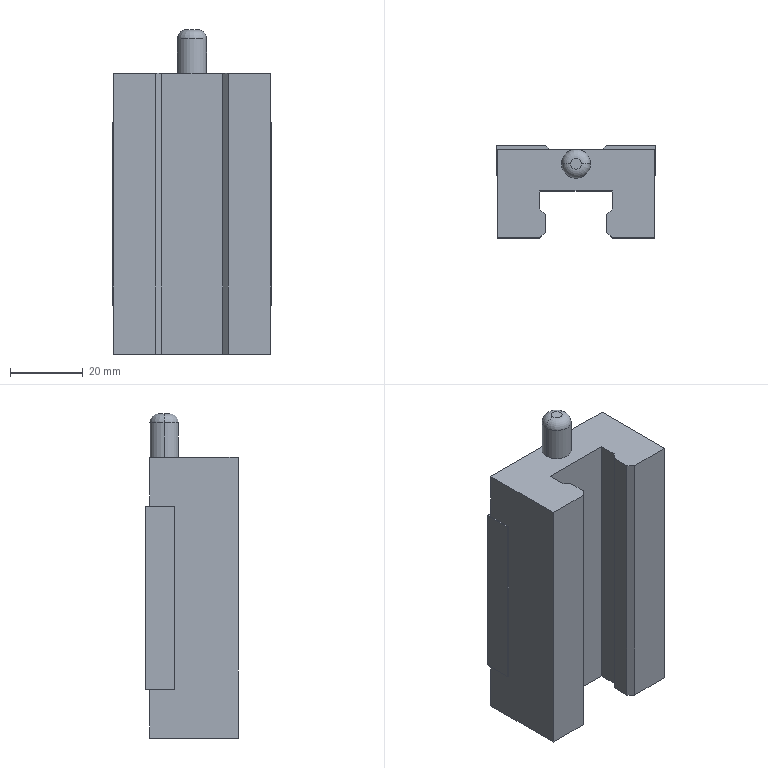Part | SolidWorks | features ICE 7, Extrusion 1, Fillet 1 | 2 solids | 52 faces | box 44 x 25.4 x 89.5 mm | volume 65459 mm3 | plane 36 | cylinder 14 | torus 2 | commonest cylinder face diameters 4.2 x8 0.1 x4 8 x2
STEP:
#1=CARTESIAN_POINT('',(16.,24.,-0.05));
#2=VERTEX_POINT('',#1);
#3=CARTESIAN_POINT('',(16.,24.,0.05));
#4=VERTEX_POINT('',#3);
#5=CARTESIAN_POINT('',(16.,24.,0.));
#6=DIRECTION('',(0.,1.,0.));
#7=DIRECTION('',(0.,0.,1.));
#8=AXIS2_PLACEMENT_3D('',#5,#6,#7);
#9=CIRCLE('',#8,0.05);
#10=EDGE_CURVE('',#2,#4,#9,.T.);
#11=ORIENTED_EDGE('',*,*,#10,.F.);
#12=CARTESIAN_POINT('',(16.,30.,-0.05));
#13=VERTEX_POINT('',#12);
#14=CARTESIAN_POINT('',(16.,24.,-0.05));
#15=DIRECTION('',(0.,1.,0.));
#16=VECTOR('',#15,1000.);
#17=LINE('',#14,#16);
#18=EDGE_CURVE('',#2,#13,#17,.T.);
#19=ORIENTED_EDGE('',*,*,#18,.T.);
#20=CARTESIAN_POINT('',(16.,30.,0.05));
#21=VERTEX_POINT('',#20);
#22=CARTESIAN_POINT('',(16.,30.,0.));
#23=DIRECTION('',(0.,1.,0.));
#24=DIRECTION('',(0.,0.,1.));
#25=AXIS2_PLACEMENT_3D('',#22,#23,#24);
#26=CIRCLE('',#25,0.05);
#27=EDGE_CURVE('',#13,#21,#26,.T.);
#28=ORIENTED_EDGE('',*,*,#27,.T.);
#29=CARTESIAN_POINT('',(16.,24.,0.05));
#30=DIRECTION('',(0.,1.,0.));
#31=VECTOR('',#30,1000.);
#32=LINE('',#29,#31);
#33=EDGE_CURVE('',#4,#21,#32,.T.);
#34=ORIENTED_EDGE('',*,*,#33,.F.);
#35=EDGE_LOOP('',(#11,#19,#28,#34));
#36=FACE_OUTER_BOUND('',#35,.T.);
#37=CARTESIAN_POINT('',(16.,24.,0.));
#38=DIRECTION('',(0.,1.,0.));
#39=DIRECTION('',(0.,0.,1.));
#40=AXIS2_PLACEMENT_3D('',#37,#38,#39);
#41=CYLINDRICAL_SURFACE('',#40,0.05);
#42=ADVANCED_FACE('',(#36),#41,.F.);
#43=CARTESIAN_POINT('',(-16.,24.,-0.05));
#44=VERTEX_POINT('',#43);
#45=CARTESIAN_POINT('',(-16.,24.,0.05));
#46=VERTEX_POINT('',#45);
#47=CARTESIAN_POINT('',(-16.,24.,0.));
#48=DIRECTION('',(0.,1.,0.));
#49=DIRECTION('',(0.,0.,1.));
#50=AXIS2_PLACEMENT_3D('',#47,#48,#49);
#51=CIRCLE('',#50,0.05);
#52=EDGE_CURVE('',#44,#46,#51,.T.);
#53=ORIENTED_EDGE('',*,*,#52,.F.);
#54=CARTESIAN_POINT('',(-16.,30.,-0.05));
#55=VERTEX_POINT('',#54);
#56=CARTESIAN_POINT('',(-16.,24.,-0.05));
#57=DIRECTION('',(0.,1.,0.));
#58=VECTOR('',#57,1000.);
#59=LINE('',#56,#58);
#60=EDGE_CURVE('',#44,#55,#59,.T.);
#61=ORIENTED_EDGE('',*,*,#60,.T.);
#62=CARTESIAN_POINT('',(-16.,30.,0.05));
#63=VERTEX_POINT('',#62);
#64=CARTESIAN_POINT('',(-16.,30.,0.));
#65=DIRECTION('',(0.,1.,0.));
#66=DIRECTION('',(0.,0.,1.));
#67=AXIS2_PLACEMENT_3D('',#64,#65,#66);
#68=CIRCLE('',#67,0.05);
#69=EDGE_CURVE('',#55,#63,#68,.T.);
#70=ORIENTED_EDGE('',*,*,#69,.T.);
#71=CARTESIAN_POINT('',(-16.,24.,0.05));
#72=DIRECTION('',(0.,1.,0.));
#73=VECTOR('',#72,1000.);
#74=LINE('',#71,#73);
#75=EDGE_CURVE('',#46,#63,#74,.T.);
#76=ORIENTED_EDGE('',*,*,#75,.F.);
#77=EDGE_LOOP('',(#53,#61,#70,#76));
#78=FACE_OUTER_BOUND('',#77,.T.);
#79=CARTESIAN_POINT('',(-16.,24.,0.));
#80=DIRECTION('',(0.,1.,0.));
#81=DIRECTION('',(0.,0.,1.));
#82=AXIS2_PLACEMENT_3D('',#79,#80,#81);
#83=CYLINDRICAL_SURFACE('',#82,0.05);
#84=ADVANCED_FACE('',(#78),#83,.F.);
#85=CARTESIAN_POINT('',(16.,24.,-20.1));
#86=VERTEX_POINT('',#85);
#87=CARTESIAN_POINT('',(16.,24.,-15.9));
#88=VERTEX_POINT('',#87);
#89=CARTESIAN_POINT('',(16.,24.,-18.));
#90=DIRECTION('',(0.,1.,0.));
#91=DIRECTION('',(0.,0.,-1.));
#92=AXIS2_PLACEMENT_3D('',#89,#90,#91);
#93=CIRCLE('',#92,2.1);
#94=EDGE_CURVE('',#86,#88,#93,.T.);
#95=ORIENTED_EDGE('',*,*,#94,.F.);
#96=CARTESIAN_POINT('',(16.,30.,-20.1));
#97=VERTEX_POINT('',#96);
#98=CARTESIAN_POINT('',(16.,24.,-20.1));
#99=DIRECTION('',(0.,1.,0.));
#100=VECTOR('',#99,1000.);
#101=LINE('',#98,#100);
#102=EDGE_CURVE('',#86,#97,#101,.T.);
#103=ORIENTED_EDGE('',*,*,#102,.T.);
#104=CARTESIAN_POINT('',(16.,30.,-15.9));
#105=VERTEX_POINT('',#104);
#106=CARTESIAN_POINT('',(16.,30.,-18.));
#107=DIRECTION('',(0.,1.,0.));
#108=DIRECTION('',(0.,0.,-1.));
#109=AXIS2_PLACEMENT_3D('',#106,#107,#108);
#110=CIRCLE('',#109,2.1);
#111=EDGE_CURVE('',#97,#105,#110,.T.);
#112=ORIENTED_EDGE('',*,*,#111,.T.);
#113=CARTESIAN_POINT('',(16.,24.,-15.9));
#114=DIRECTION('',(0.,1.,0.));
#115=VECTOR('',#114,1000.);
#116=LINE('',#113,#115);
#117=EDGE_CURVE('',#88,#105,#116,.T.);
#118=ORIENTED_EDGE('',*,*,#117,.F.);
#119=EDGE_LOOP('',(#95,#103,#112,#118));
#120=FACE_OUTER_BOUND('',#119,.T.);
#121=CARTESIAN_POINT('',(16.,24.,-18.));
#122=DIRECTION('',(0.,1.,0.));
#123=DIRECTION('',(0.,0.,1.));
#124=AXIS2_PLACEMENT_3D('',#121,#122,#123);
#125=CYLINDRICAL_SURFACE('',#124,2.1);
#126=ADVANCED_FACE('',(#120),#125,.F.);
#127=CARTESIAN_POINT('',(-16.,24.,-20.1));
#128=VERTEX_POINT('',#127);
#129=CARTESIAN_POINT('',(-16.,24.,-15.9));
#130=VERTEX_POINT('',#129);
#131=CARTESIAN_POINT('',(-16.,24.,-18.));
#132=DIRECTION('',(0.,1.,0.));
#133=DIRECTION('',(0.,0.,-1.));
#134=AXIS2_PLACEMENT_3D('',#131,#132,#133);
#135=CIRCLE('',#134,2.1);
#136=EDGE_CURVE('',#128,#130,#135,.T.);
#137=ORIENTED_EDGE('',*,*,#136,.F.);
#138=CARTESIAN_POINT('',(-16.,30.,-20.1));
#139=VERTEX_POINT('',#138);
#140=CARTESIAN_POINT('',(-16.,24.,-20.1));
#141=DIRECTION('',(0.,1.,0.));
#142=VECTOR('',#141,1000.);
#143=LINE('',#140,#142);
#144=EDGE_CURVE('',#128,#139,#143,.T.);
#145=ORIENTED_EDGE('',*,*,#144,.T.);
#146=CARTESIAN_POINT('',(-16.,30.,-15.9));
#147=VERTEX_POINT('',#146);
#148=CARTESIAN_POINT('',(-16.,30.,-18.));
#149=DIRECTION('',(0.,1.,0.));
#150=DIRECTION('',(0.,0.,-1.));
#151=AXIS2_PLACEMENT_3D('',#148,#149,#150);
#152=CIRCLE('',#151,2.1);
#153=EDGE_CURVE('',#139,#147,#152,.T.);
#154=ORIENTED_EDGE('',*,*,#153,.T.);
#155=CARTESIAN_POINT('',(-16.,24.,-15.9));
#156=DIRECTION('',(0.,1.,0.));
#157=VECTOR('',#156,1000.);
#158=LINE('',#155,#157);
#159=EDGE_CURVE('',#130,#147,#158,.T.);
#160=ORIENTED_EDGE('',*,*,#159,.F.);
#161=EDGE_LOOP('',(#137,#145,#154,#160));
#162=FACE_OUTER_BOUND('',#161,.T.);
#163=CARTESIAN_POINT('',(-16.,24.,-18.));
#164=DIRECTION('',(0.,1.,0.));
#165=DIRECTION('',(0.,0.,1.));
#166=AXIS2_PLACEMENT_3D('',#163,#164,#165);
#167=CYLINDRICAL_SURFACE('',#166,2.1);
#168=ADVANCED_FACE('',(#162),#167,.F.);
#169=CARTESIAN_POINT('',(-16.,24.,15.9));
#170=VERTEX_POINT('',#169);
#171=CARTESIAN_POINT('',(-16.,24.,20.1));
#172=VERTEX_POINT('',#171);
#173=CARTESIAN_POINT('',(-16.,24.,18.));
#174=DIRECTION('',(0.,1.,0.));
#175=DIRECTION('',(0.,0.,1.));
#176=AXIS2_PLACEMENT_3D('',#173,#174,#175);
#177=CIRCLE('',#176,2.1);
#178=EDGE_CURVE('',#170,#172,#177,.T.);
#179=ORIENTED_EDGE('',*,*,#178,.F.);
#180=CARTESIAN_POINT('',(-16.,30.,15.9));
#181=VERTEX_POINT('',#180);
#182=CARTESIAN_POINT('',(-16.,24.,15.9));
#183=DIRECTION('',(0.,1.,0.));
#184=VECTOR('',#183,1000.);
#185=LINE('',#182,#184);
#186=EDGE_CURVE('',#170,#181,#185,.T.);
#187=ORIENTED_EDGE('',*,*,#186,.T.);
#188=CARTESIAN_POINT('',(-16.,30.,20.1));
#189=VERTEX_POINT('',#188);
#190=CARTESIAN_POINT('',(-16.,30.,18.));
#191=DIRECTION('',(0.,1.,0.));
#192=DIRECTION('',(0.,0.,1.));
#193=AXIS2_PLACEMENT_3D('',#190,#191,#192);
#194=CIRCLE('',#193,2.1);
#195=EDGE_CURVE('',#181,#189,#194,.T.);
#196=ORIENTED_EDGE('',*,*,#195,.T.);
#197=CARTESIAN_POINT('',(-16.,24.,20.1));
#198=DIRECTION('',(0.,1.,0.));
#199=VECTOR('',#198,1000.);
#200=LINE('',#197,#199);
#201=EDGE_CURVE('',#172,#189,#200,.T.);
#202=ORIENTED_EDGE('',*,*,#201,.F.);
#203=EDGE_LOOP('',(#179,#187,#196,#202));
#204=FACE_OUTER_BOUND('',#203,.T.);
#205=CARTESIAN_POINT('',(-16.,24.,18.));
#206=DIRECTION('',(0.,1.,0.));
#207=DIRECTION('',(0.,0.,1.));
#208=AXIS2_PLACEMENT_3D('',#205,#206,#207);
#209=CYLINDRICAL_SURFACE('',#208,2.1);
#210=ADVANCED_FACE('',(#204),#209,.F.);
#211=CARTESIAN_POINT('',(16.,24.,15.9));
#212=VERTEX_POINT('',#211);
#213=CARTESIAN_POINT('',(16.,24.,20.1));
#214=VERTEX_POINT('',#213);
#215=CARTESIAN_POINT('',(16.,24.,18.));
#216=DIRECTION('',(0.,1.,0.));
#217=DIRECTION('',(0.,0.,1.));
#218=AXIS2_PLACEMENT_3D('',#215,#216,#217);
#219=CIRCLE('',#218,2.1);
#220=EDGE_CURVE('',#212,#214,#219,.T.);
#221=ORIENTED_EDGE('',*,*,#220,.F.);
#222=CARTESIAN_POINT('',(16.,30.,15.9));
#223=VERTEX_POINT('',#222);
#224=CARTESIAN_POINT('',(16.,24.,15.9));
#225=DIRECTION('',(0.,1.,0.));
#226=VECTOR('',#225,1000.);
#227=LINE('',#224,#226);
#228=EDGE_CURVE('',#212,#223,#227,.T.);
#229=ORIENTED_EDGE('',*,*,#228,.T.);
#230=CARTESIAN_POINT('',(16.,30.,20.1));
#231=VERTEX_POINT('',#230);
#232=CARTESIAN_POINT('',(16.,30.,18.));
#233=DIRECTION('',(0.,1.,0.));
#234=DIRECTION('',(0.,0.,1.));
#235=AXIS2_PLACEMENT_3D('',#232,#233,#234);
#236=CIRCLE('',#235,2.1);
#237=EDGE_CURVE('',#223,#231,#236,.T.);
#238=ORIENTED_EDGE('',*,*,#237,.T.);
#239=CARTESIAN_POINT('',(16.,24.,20.1));
#240=DIRECTION('',(0.,1.,0.));
#241=VECTOR('',#240,1000.);
#242=LINE('',#239,#241);
#243=EDGE_CURVE('',#214,#231,#242,.T.);
#244=ORIENTED_EDGE('',*,*,#243,.F.);
#245=EDGE_LOOP('',(#221,#229,#238,#244));
#246=FACE_OUTER_BOUND('',#245,.T.);
#247=CARTESIAN_POINT('',(16.,24.,18.));
#248=DIRECTION('',(0.,1.,0.));
#249=DIRECTION('',(0.,0.,1.));
#250=AXIS2_PLACEMENT_3D('',#247,#248,#249);
#251=CYLINDRICAL_SURFACE('',#250,2.1);
#252=ADVANCED_FACE('',(#246),#251,.F.);
#253=CARTESIAN_POINT('',(-16.,30.,18.));
#254=DIRECTION('',(0.,1.,0.));
#255=DIRECTION('',(0.,0.,1.));
#256=AXIS2_PLACEMENT_3D('',#253,#254,#255);
#257=CIRCLE('',#256,2.1);
#258=EDGE_CURVE('',#189,#181,#257,.T.);
#259=ORIENTED_EDGE('',*,*,#258,.F.);
#260=ORIENTED_EDGE('',*,*,#195,.F.);
#261=EDGE_LOOP('',(#259,#260));
#262=FACE_BOUND('',#261,.T.);
#263=CARTESIAN_POINT('',(-16.,30.,-18.));
#264=DIRECTION('',(0.,1.,0.));
#265=DIRECTION('',(0.,0.,-1.));
#266=AXIS2_PLACEMENT_3D('',#263,#264,#265);
#267=CIRCLE('',#266,2.1);
#268=EDGE_CURVE('',#147,#139,#267,.T.);
#269=ORIENTED_EDGE('',*,*,#268,.F.);
#270=ORIENTED_EDGE('',*,*,#153,.F.);
#271=EDGE_LOOP('',(#269,#270));
#272=FACE_BOUND('',#271,.T.);
#273=CARTESIAN_POINT('',(-16.,30.,0.));
#274=DIRECTION('',(0.,1.,0.));
#275=DIRECTION('',(0.,0.,1.));
#276=AXIS2_PLACEMENT_3D('',#273,#274,#275);
#277=CIRCLE('',#276,0.05);
#278=EDGE_CURVE('',#63,#55,#277,.T.);
#279=ORIENTED_EDGE('',*,*,#278,.F.);
#280=ORIENTED_EDGE('',*,*,#69,.F.);
#281=EDGE_LOOP('',(#279,#280));
#282=FACE_BOUND('',#281,.T.);
#283=CARTESIAN_POINT('',(-8.333,30.,25.25));
#284=VERTEX_POINT('',#283);
#285=CARTESIAN_POINT('',(-22.,30.,25.25));
#286=VERTEX_POINT('',#285);
#287=CARTESIAN_POINT('',(-22.,30.,25.25));
#288=DIRECTION('',(-1.,0.,0.));
#289=VECTOR('',#288,1000.);
#290=LINE('',#287,#289);
#291=EDGE_CURVE('',#284,#286,#290,.T.);
#292=ORIENTED_EDGE('',*,*,#291,.F.);
#293=CARTESIAN_POINT('',(-8.333,30.,-25.25));
#294=VERTEX_POINT('',#293);
#295=CARTESIAN_POINT('',(-8.333,30.,-38.75));
#296=DIRECTION('',(0.,0.,1.));
#297=VECTOR('',#296,1000.);
#298=LINE('',#295,#297);
#299=EDGE_CURVE('',#294,#284,#298,.T.);
#300=ORIENTED_EDGE('',*,*,#299,.F.);
#301=CARTESIAN_POINT('',(-22.,30.,-25.25));
#302=VERTEX_POINT('',#301);
#303=CARTESIAN_POINT('',(22.,30.,-25.25));
#304=DIRECTION('',(1.,0.,0.));
#305=VECTOR('',#304,1000.);
#306=LINE('',#303,#305);
#307=EDGE_CURVE('',#302,#294,#306,.T.);
#308=ORIENTED_EDGE('',*,*,#307,.F.);
#309=CARTESIAN_POINT('',(-22.,30.,38.75));
#310=DIRECTION('',(0.,0.,-1.));
#311=VECTOR('',#310,1000.);
#312=LINE('',#309,#311);
#313=EDGE_CURVE('',#286,#302,#312,.T.);
#314=ORIENTED_EDGE('',*,*,#313,.F.);
#315=EDGE_LOOP('',(#292,#300,#308,#314));
#316=FACE_OUTER_BOUND('',#315,.T.);
#317=CARTESIAN_POINT('',(-22.,30.,38.75));
#318=DIRECTION('',(0.,-1.,0.));
#319=DIRECTION('',(0.,0.,-1.));
#320=AXIS2_PLACEMENT_3D('',#317,#318,#319);
#321=PLANE('',#320);
#322=ADVANCED_FACE('',(#262,#272,#282,#316),#321,.F.);
#323=CARTESIAN_POINT('',(-21.7,29.,25.25));
#324=VERTEX_POINT('',#323);
#325=CARTESIAN_POINT('',(-7.333,29.,25.25));
#326=VERTEX_POINT('',#325);
#327=CARTESIAN_POINT('',(-22.,29.,25.25));
#328=DIRECTION('',(1.,0.,0.));
#329=VECTOR('',#328,1000.);
#330=LINE('',#327,#329);
#331=EDGE_CURVE('',#324,#326,#330,.T.);
#332=ORIENTED_EDGE('',*,*,#331,.T.);
#333=CARTESIAN_POINT('',(-2.467,24.133,25.25));
#334=DIRECTION('',(-0.7071,0.7071,0.));
#335=VECTOR('',#334,1000.);
#336=LINE('',#333,#335);
#337=EDGE_CURVE('',#326,#284,#336,.T.);
#338=ORIENTED_EDGE('',*,*,#337,.T.);
#339=ORIENTED_EDGE('',*,*,#291,.T.);
#340=CARTESIAN_POINT('',(-22.,22.,25.25));
#341=VERTEX_POINT('',#340);
#342=CARTESIAN_POINT('',(-22.,4.6,25.25));
#343=DIRECTION('',(0.,1.,0.));
#344=VECTOR('',#343,1000.);
#345=LINE('',#342,#344);
#346=EDGE_CURVE('',#341,#286,#345,.T.);
#347=ORIENTED_EDGE('',*,*,#346,.F.);
#348=CARTESIAN_POINT('',(-21.7,22.,25.25));
#349=VERTEX_POINT('',#348);
#350=CARTESIAN_POINT('',(-21.7,22.,25.25));
#351=DIRECTION('',(-1.,0.,0.));
#352=VECTOR('',#351,1000.);
#353=LINE('',#350,#352);
#354=EDGE_CURVE('',#349,#341,#353,.T.);
#355=ORIENTED_EDGE('',*,*,#354,.F.);
#356=CARTESIAN_POINT('',(-21.7,4.6,25.25));
#357=DIRECTION('',(0.,1.,0.));
#358=VECTOR('',#357,1000.);
#359=LINE('',#356,#358);
#360=EDGE_CURVE('',#349,#324,#359,.T.);
#361=ORIENTED_EDGE('',*,*,#360,.T.);
#362=EDGE_LOOP('',(#332,#338,#339,#347,#355,#361));
#363=FACE_OUTER_BOUND('',#362,.T.);
#364=CARTESIAN_POINT('',(-22.,4.6,25.25));
#365=DIRECTION('',(0.,0.,-1.));
#366=DIRECTION('',(-1.,0.,0.));
#367=AXIS2_PLACEMENT_3D('',#364,#365,#366);
#368=PLANE('',#367);
#369=ADVANCED_FACE('',(#363),#368,.F.);
#370=ORIENTED_EDGE('',*,*,#307,.T.);
#371=CARTESIAN_POINT('',(-7.333,29.,-25.25));
#372=VERTEX_POINT('',#371);
#373=CARTESIAN_POINT('',(19.533,2.133,-25.25));
#374=DIRECTION('',(0.7071,-0.7071,0.));
#375=VECTOR('',#374,1000.);
#376=LINE('',#373,#375);
#377=EDGE_CURVE('',#294,#372,#376,.T.);
#378=ORIENTED_EDGE('',*,*,#377,.T.);
#379=CARTESIAN_POINT('',(-21.7,29.,-25.25));
#380=VERTEX_POINT('',#379);
#381=CARTESIAN_POINT('',(-22.,29.,-25.25));
#382=DIRECTION('',(1.,0.,0.));
#383=VECTOR('',#382,1000.);
#384=LINE('',#381,#383);
#385=EDGE_CURVE('',#380,#372,#384,.T.);
#386=ORIENTED_EDGE('',*,*,#385,.F.);
#387=CARTESIAN_POINT('',(-21.7,22.,-25.25));
#388=VERTEX_POINT('',#387);
#389=CARTESIAN_POINT('',(-21.7,4.6,-25.25));
#390=DIRECTION('',(0.,1.,0.));
#391=VECTOR('',#390,1000.);
#392=LINE('',#389,#391);
#393=EDGE_CURVE('',#388,#380,#392,.T.);
#394=ORIENTED_EDGE('',*,*,#393,.F.);
#395=CARTESIAN_POINT('',(-22.,22.,-25.25));
#396=VERTEX_POINT('',#395);
#397=CARTESIAN_POINT('',(-21.7,22.,-25.25));
#398=DIRECTION('',(1.,0.,0.));
#399=VECTOR('',#398,1000.);
#400=LINE('',#397,#399);
#401=EDGE_CURVE('',#396,#388,#400,.T.);
#402=ORIENTED_EDGE('',*,*,#401,.F.);
#403=CARTESIAN_POINT('',(-22.,4.6,-25.25));
#404=DIRECTION('',(0.,1.,0.));
#405=VECTOR('',#404,1000.);
#406=LINE('',#403,#405);
#407=EDGE_CURVE('',#396,#302,#406,.T.);
#408=ORIENTED_EDGE('',*,*,#407,.T.);
#409=EDGE_LOOP('',(#370,#378,#386,#394,#402,#408));
#410=FACE_OUTER_BOUND('',#409,.T.);
#411=CARTESIAN_POINT('',(22.,4.6,-25.25));
#412=DIRECTION('',(0.,0.,1.));
#413=DIRECTION('',(1.,0.,0.));
#414=AXIS2_PLACEMENT_3D('',#411,#412,#413);
#415=PLANE('',#414);
#416=ADVANCED_FACE('',(#410),#415,.F.);
#417=CARTESIAN_POINT('',(16.,30.,0.));
#418=DIRECTION('',(0.,1.,0.));
#419=DIRECTION('',(0.,0.,1.));
#420=AXIS2_PLACEMENT_3D('',#417,#418,#419);
#421=CIRCLE('',#420,0.05);
#422=EDGE_CURVE('',#21,#13,#421,.T.);
#423=ORIENTED_EDGE('',*,*,#422,.F.);
#424=ORIENTED_EDGE('',*,*,#27,.F.);
#425=EDGE_LOOP('',(#423,#424));
#426=FACE_BOUND('',#425,.T.);
#427=CARTESIAN_POINT('',(16.,30.,-18.));
#428=DIRECTION('',(0.,1.,0.));
#429=DIRECTION('',(0.,0.,-1.));
#430=AXIS2_PLACEMENT_3D('',#427,#428,#429);
#431=CIRCLE('',#430,2.1);
#432=EDGE_CURVE('',#105,#97,#431,.T.);
#433=ORIENTED_EDGE('',*,*,#432,.F.);
#434=ORIENTED_EDGE('',*,*,#111,.F.);
#435=EDGE_LOOP('',(#433,#434));
#436=FACE_BOUND('',#435,.T.);
#437=CARTESIAN_POINT('',(16.,30.,18.));
#438=DIRECTION('',(0.,1.,0.));
#439=DIRECTION('',(0.,0.,1.));
#440=AXIS2_PLACEMENT_3D('',#437,#438,#439);
#441=CIRCLE('',#440,2.1);
#442=EDGE_CURVE('',#231,#223,#441,.T.);
#443=ORIENTED_EDGE('',*,*,#442,.F.);
#444=ORIENTED_EDGE('',*,*,#237,.F.);
#445=EDGE_LOOP('',(#443,#444));
#446=FACE_BOUND('',#445,.T.);
#447=CARTESIAN_POINT('',(8.333,30.,-25.25));
#448=VERTEX_POINT('',#447);
#449=CARTESIAN_POINT('',(22.,30.,-25.25));
#450=VERTEX_POINT('',#449);
#451=CARTESIAN_POINT('',(22.,30.,-25.25));
#452=DIRECTION('',(1.,0.,0.));
#453=VECTOR('',#452,1000.);
#454=LINE('',#451,#453);
#455=EDGE_CURVE('',#448,#450,#454,.T.);
#456=ORIENTED_EDGE('',*,*,#455,.F.);
#457=CARTESIAN_POINT('',(8.333,30.,25.25));
#458=VERTEX_POINT('',#457);
#459=CARTESIAN_POINT('',(8.333,30.,-38.75));
#460=DIRECTION('',(0.,0.,1.));
#461=VECTOR('',#460,1000.);
#462=LINE('',#459,#461);
#463=EDGE_CURVE('',#448,#458,#462,.T.);
#464=ORIENTED_EDGE('',*,*,#463,.T.);
#465=CARTESIAN_POINT('',(22.,30.,25.25));
#466=VERTEX_POINT('',#465);
#467=CARTESIAN_POINT('',(-22.,30.,25.25));
#468=DIRECTION('',(-1.,0.,0.));
#469=VECTOR('',#468,1000.);
#470=LINE('',#467,#469);
#471=EDGE_CURVE('',#466,#458,#470,.T.);
#472=ORIENTED_EDGE('',*,*,#471,.F.);
#473=CARTESIAN_POINT('',(22.,30.,38.75));
#474=DIRECTION('',(0.,0.,-1.));
#475=VECTOR('',#474,1000.);
#476=LINE('',#473,#475);
#477=EDGE_CURVE('',#466,#450,#476,.T.);
#478=ORIENTED_EDGE('',*,*,#477,.T.);
#479=EDGE_LOOP('',(#456,#464,#472,#478));
#480=FACE_OUTER_BOUND('',#479,.T.);
#481=CARTESIAN_POINT('',(-22.,30.,38.75));
#482=DIRECTION('',(0.,-1.,0.));
#483=DIRECTION('',(0.,0.,-1.));
#484=AXIS2_PLACEMENT_3D('',#481,#482,#483);
#485=PLANE('',#484);
#486=ADVANCED_FACE('',(#426,#436,#446,#480),#485,.F.);
#487=ORIENTED_EDGE('',*,*,#313,.T.);
#488=ORIENTED_EDGE('',*,*,#407,.F.);
#489=CARTESIAN_POINT('',(-22.,22.,-38.75));
#490=DIRECTION('',(0.,0.,1.));
#491=VECTOR('',#490,1000.);
#492=LINE('',#489,#491);
#493=EDGE_CURVE('',#396,#341,#492,.T.);
#494=ORIENTED_EDGE('',*,*,#493,.T.);
#495=ORIENTED_EDGE('',*,*,#346,.T.);
#496=EDGE_LOOP('',(#487,#488,#494,#495));
#497=FACE_OUTER_BOUND('',#496,.T.);
#498=CARTESIAN_POINT('',(-22.,4.6,38.75));
#499=DIRECTION('',(1.,0.,0.));
#500=DIRECTION('',(0.,1.,0.));
#501=AXIS2_PLACEMENT_3D('',#498,#499,#500);
#502=PLANE('',#501);
#503=ADVANCED_FACE('',(#497),#502,.F.);
#504=CARTESIAN_POINT('',(-21.7,4.6,38.75));
#505=VERTEX_POINT('',#504);
#506=CARTESIAN_POINT('',(-10.,4.6,38.75));
#507=VERTEX_POINT('',#506);
#508=CARTESIAN_POINT('',(-10.,4.6,38.75));
#509=DIRECTION('',(1.,0.,0.));
#510=VECTOR('',#509,1000.);
#511=LINE('',#508,#510);
#512=EDGE_CURVE('',#505,#507,#511,.T.);
#513=ORIENTED_EDGE('',*,*,#512,.F.);
#514=CARTESIAN_POINT('',(-21.7,4.6,-38.75));
#515=VERTEX_POINT('',#514);
#516=CARTESIAN_POINT('',(-21.7,4.6,-38.75));
#517=DIRECTION('',(0.,0.,1.));
#518=VECTOR('',#517,1000.);
#519=LINE('',#516,#518);
#520=EDGE_CURVE('',#515,#505,#519,.T.);
#521=ORIENTED_EDGE('',*,*,#520,.F.);
#522=CARTESIAN_POINT('',(-10.,4.6,-38.75));
#523=VERTEX_POINT('',#522);
#524=CARTESIAN_POINT('',(-10.,4.6,-38.75));
#525=DIRECTION('',(1.,0.,0.));
#526=VECTOR('',#525,1000.);
#527=LINE('',#524,#526);
#528=EDGE_CURVE('',#515,#523,#527,.T.);
#529=ORIENTED_EDGE('',*,*,#528,.T.);
#530=CARTESIAN_POINT('',(-10.,4.6,38.75));
#531=DIRECTION('',(0.,0.,-1.));
#532=VECTOR('',#531,1000.);
#533=LINE('',#530,#532);
#534=EDGE_CURVE('',#507,#523,#533,.T.);
#535=ORIENTED_EDGE('',*,*,#534,.F.);
#536=EDGE_LOOP('',(#513,#521,#529,#535));
#537=FACE_OUTER_BOUND('',#536,.T.);
#538=CARTESIAN_POINT('',(-10.,4.6,38.75));
#539=DIRECTION('',(0.,1.,0.));
#540=DIRECTION('',(0.,0.,1.));
#541=AXIS2_PLACEMENT_3D('',#538,#539,#540);
#542=PLANE('',#541);
#543=ADVANCED_FACE('',(#537),#542,.F.);
#544=CARTESIAN_POINT('',(-8.5,6.1,-38.75));
#545=VERTEX_POINT('',#544);
#546=CARTESIAN_POINT('',(-10.,4.6,-38.75));
#547=DIRECTION('',(0.7071,0.7071,0.));
#548=VECTOR('',#547,1000.);
#549=LINE('',#546,#548);
#550=EDGE_CURVE('',#523,#545,#549,.T.);
#551=ORIENTED_EDGE('',*,*,#550,.T.);
#552=CARTESIAN_POINT('',(-8.5,6.1,38.75));
#553=VERTEX_POINT('',#552);
#554=CARTESIAN_POINT('',(-8.5,6.1,38.75));
#555=DIRECTION('',(0.,0.,-1.));
#556=VECTOR('',#555,1000.);
#557=LINE('',#554,#556);
#558=EDGE_CURVE('',#553,#545,#557,.T.);
#559=ORIENTED_EDGE('',*,*,#558,.F.);
#560=CARTESIAN_POINT('',(-10.,4.6,38.75));
#561=DIRECTION('',(0.7071,0.7071,0.));
#562=VECTOR('',#561,1000.);
#563=LINE('',#560,#562);
#564=EDGE_CURVE('',#507,#553,#563,.T.);
#565=ORIENTED_EDGE('',*,*,#564,.F.);
#566=ORIENTED_EDGE('',*,*,#534,.T.);
#567=EDGE_LOOP('',(#551,#559,#565,#566));
#568=FACE_OUTER_BOUND('',#567,.T.);
#569=CARTESIAN_POINT('',(-10.,4.6,38.75));
#570=DIRECTION('',(-0.7071,0.7071,0.));
#571=DIRECTION('',(-0.7071,-0.7071,0.));
#572=AXIS2_PLACEMENT_3D('',#569,#570,#571);
#573=PLANE('',#572);
#574=ADVANCED_FACE('',(#568),#573,.F.);
#575=CARTESIAN_POINT('',(-8.5,11.05,-38.75));
#576=VERTEX_POINT('',#575);
#577=CARTESIAN_POINT('',(-8.5,6.1,-38.75));
#578=DIRECTION('',(0.,1.,0.));
#579=VECTOR('',#578,1000.);
#580=LINE('',#577,#579);
#581=EDGE_CURVE('',#545,#576,#580,.T.);
#582=ORIENTED_EDGE('',*,*,#581,.T.);
#583=CARTESIAN_POINT('',(-8.5,11.05,38.75));
#584=VERTEX_POINT('',#583);
#585=CARTESIAN_POINT('',(-8.5,11.05,38.75));
#586=DIRECTION('',(0.,0.,-1.));
#587=VECTOR('',#586,1000.);
#588=LINE('',#585,#587);
#589=EDGE_CURVE('',#584,#576,#588,.T.);
#590=ORIENTED_EDGE('',*,*,#589,.F.);
#591=CARTESIAN_POINT('',(-8.5,6.1,38.75));
#592=DIRECTION('',(0.,1.,0.));
#593=VECTOR('',#592,1000.);
#594=LINE('',#591,#593);
#595=EDGE_CURVE('',#553,#584,#594,.T.);
#596=ORIENTED_EDGE('',*,*,#595,.F.);
#597=ORIENTED_EDGE('',*,*,#558,.T.);
#598=EDGE_LOOP('',(#582,#590,#596,#597));
#599=FACE_OUTER_BOUND('',#598,.T.);
#600=CARTESIAN_POINT('',(-8.5,6.1,38.75));
#601=DIRECTION('',(-1.,0.,0.));
#602=DIRECTION('',(0.,0.,1.));
#603=AXIS2_PLACEMENT_3D('',#600,#601,#602);
#604=PLANE('',#603);
#605=ADVANCED_FACE('',(#599),#604,.F.);
#606=CARTESIAN_POINT('',(-10.,12.55,-38.75));
#607=VERTEX_POINT('',#606);
#608=CARTESIAN_POINT('',(-8.5,11.05,-38.75));
#609=DIRECTION('',(-0.7071,0.7071,0.));
#610=VECTOR('',#609,1000.);
#611=LINE('',#608,#610);
#612=EDGE_CURVE('',#576,#607,#611,.T.);
#613=ORIENTED_EDGE('',*,*,#612,.T.);
#614=CARTESIAN_POINT('',(-10.,12.55,38.75));
#615=VERTEX_POINT('',#614);
#616=CARTESIAN_POINT('',(-10.,12.55,38.75));
#617=DIRECTION('',(0.,0.,-1.));
#618=VECTOR('',#617,1000.);
#619=LINE('',#616,#618);
#620=EDGE_CURVE('',#615,#607,#619,.T.);
#621=ORIENTED_EDGE('',*,*,#620,.F.);
#622=CARTESIAN_POINT('',(-8.5,11.05,38.75));
#623=DIRECTION('',(-0.7071,0.7071,0.));
#624=VECTOR('',#623,1000.);
#625=LINE('',#622,#624);
#626=EDGE_CURVE('',#584,#615,#625,.T.);
#627=ORIENTED_EDGE('',*,*,#626,.F.);
#628=ORIENTED_EDGE('',*,*,#589,.T.);
#629=EDGE_LOOP('',(#613,#621,#627,#628));
#630=FACE_OUTER_BOUND('',#629,.T.);
#631=CARTESIAN_POINT('',(-8.5,11.05,38.75));
#632=DIRECTION('',(-0.7071,-0.7071,0.));
#633=DIRECTION('',(0.7071,-0.7071,0.));
#634=AXIS2_PLACEMENT_3D('',#631,#632,#633);
#635=PLANE('',#634);
#636=ADVANCED_FACE('',(#630),#635,.F.);
#637=CARTESIAN_POINT('',(-10.,17.5,-38.75));
#638=VERTEX_POINT('',#637);
#639=CARTESIAN_POINT('',(-10.,12.55,-38.75));
#640=DIRECTION('',(0.,1.,0.));
#641=VECTOR('',#640,1000.);
#642=LINE('',#639,#641);
#643=EDGE_CURVE('',#607,#638,#642,.T.);
#644=ORIENTED_EDGE('',*,*,#643,.T.);
#645=CARTESIAN_POINT('',(-10.,17.5,38.75));
#646=VERTEX_POINT('',#645);
#647=CARTESIAN_POINT('',(-10.,17.5,38.75));
#648=DIRECTION('',(0.,0.,-1.));
#649=VECTOR('',#648,1000.);
#650=LINE('',#647,#649);
#651=EDGE_CURVE('',#646,#638,#650,.T.);
#652=ORIENTED_EDGE('',*,*,#651,.F.);
#653=CARTESIAN_POINT('',(-10.,12.55,38.75));
#654=DIRECTION('',(0.,1.,0.));
#655=VECTOR('',#654,1000.);
#656=LINE('',#653,#655);
#657=EDGE_CURVE('',#615,#646,#656,.T.);
#658=ORIENTED_EDGE('',*,*,#657,.F.);
#659=ORIENTED_EDGE('',*,*,#620,.T.);
#660=EDGE_LOOP('',(#644,#652,#658,#659));
#661=FACE_OUTER_BOUND('',#660,.T.);
#662=CARTESIAN_POINT('',(-10.,12.55,38.75));
#663=DIRECTION('',(-1.,0.,0.));
#664=DIRECTION('',(0.,0.,1.));
#665=AXIS2_PLACEMENT_3D('',#662,#663,#664);
#666=PLANE('',#665);
#667=ADVANCED_FACE('',(#661),#666,.F.);
#668=CARTESIAN_POINT('',(10.,17.5,-38.75));
#669=VERTEX_POINT('',#668);
#670=CARTESIAN_POINT('',(-10.,17.5,-38.75));
#671=DIRECTION('',(1.,0.,0.));
#672=VECTOR('',#671,1000.);
#673=LINE('',#670,#672);
#674=EDGE_CURVE('',#638,#669,#673,.T.);
#675=ORIENTED_EDGE('',*,*,#674,.T.);
#676=CARTESIAN_POINT('',(10.,17.5,38.75));
#677=VERTEX_POINT('',#676);
#678=CARTESIAN_POINT('',(10.,17.5,38.75));
#679=DIRECTION('',(0.,0.,-1.));
#680=VECTOR('',#679,1000.);
#681=LINE('',#678,#680);
#682=EDGE_CURVE('',#677,#669,#681,.T.);
#683=ORIENTED_EDGE('',*,*,#682,.F.);
#684=CARTESIAN_POINT('',(-10.,17.5,38.75));
#685=DIRECTION('',(1.,0.,0.));
#686=VECTOR('',#685,1000.);
#687=LINE('',#684,#686);
#688=EDGE_CURVE('',#646,#677,#687,.T.);
#689=ORIENTED_EDGE('',*,*,#688,.F.);
#690=ORIENTED_EDGE('',*,*,#651,.T.);
#691=EDGE_LOOP('',(#675,#683,#689,#690));
#692=FACE_OUTER_BOUND('',#691,.T.);
#693=CARTESIAN_POINT('',(-10.,17.5,38.75));
#694=DIRECTION('',(0.,1.,0.));
#695=DIRECTION('',(0.,0.,1.));
#696=AXIS2_PLACEMENT_3D('',#693,#694,#695);
#697=PLANE('',#696);
#698=ADVANCED_FACE('',(#692),#697,.F.);
#699=CARTESIAN_POINT('',(10.,12.55,-38.75));
#700=VERTEX_POINT('',#699);
#701=CARTESIAN_POINT('',(10.,12.55,-38.75));
#702=DIRECTION('',(0.,-1.,0.));
#703=VECTOR('',#702,1000.);
#704=LINE('',#701,#703);
#705=EDGE_CURVE('',#669,#700,#704,.T.);
#706=ORIENTED_EDGE('',*,*,#705,.T.);
#707=CARTESIAN_POINT('',(10.,12.55,38.75));
#708=VERTEX_POINT('',#707);
#709=CARTESIAN_POINT('',(10.,12.55,38.75));
#710=DIRECTION('',(0.,0.,-1.));
#711=VECTOR('',#710,1000.);
#712=LINE('',#709,#711);
#713=EDGE_CURVE('',#708,#700,#712,.T.);
#714=ORIENTED_EDGE('',*,*,#713,.F.);
#715=CARTESIAN_POINT('',(10.,12.55,38.75));
#716=DIRECTION('',(0.,-1.,0.));
#717=VECTOR('',#716,1000.);
#718=LINE('',#715,#717);
#719=EDGE_CURVE('',#677,#708,#718,.T.);
#720=ORIENTED_EDGE('',*,*,#719,.F.);
#721=ORIENTED_EDGE('',*,*,#682,.T.);
#722=EDGE_LOOP('',(#706,#714,#720,#721));
#723=FACE_OUTER_BOUND('',#722,.T.);
#724=CARTESIAN_POINT('',(10.,12.55,38.75));
#725=DIRECTION('',(1.,0.,0.));
#726=DIRECTION('',(0.,0.,-1.));
#727=AXIS2_PLACEMENT_3D('',#724,#725,#726);
#728=PLANE('',#727);
#729=ADVANCED_FACE('',(#723),#728,.F.);
#730=CARTESIAN_POINT('',(8.5,11.05,-38.75));
#731=VERTEX_POINT('',#730);
#732=CARTESIAN_POINT('',(8.5,11.05,-38.75));
#733=DIRECTION('',(-0.7071,-0.7071,0.));
#734=VECTOR('',#733,1000.);
#735=LINE('',#732,#734);
#736=EDGE_CURVE('',#700,#731,#735,.T.);
#737=ORIENTED_EDGE('',*,*,#736,.T.);
#738=CARTESIAN_POINT('',(8.5,11.05,38.75));
#739=VERTEX_POINT('',#738);
#740=CARTESIAN_POINT('',(8.5,11.05,38.75));
#741=DIRECTION('',(0.,0.,-1.));
#742=VECTOR('',#741,1000.);
#743=LINE('',#740,#742);
#744=EDGE_CURVE('',#739,#731,#743,.T.);
#745=ORIENTED_EDGE('',*,*,#744,.F.);
#746=CARTESIAN_POINT('',(8.5,11.05,38.75));
#747=DIRECTION('',(-0.7071,-0.7071,0.));
#748=VECTOR('',#747,1000.);
#749=LINE('',#746,#748);
#750=EDGE_CURVE('',#708,#739,#749,.T.);
#751=ORIENTED_EDGE('',*,*,#750,.F.);
#752=ORIENTED_EDGE('',*,*,#713,.T.);
#753=EDGE_LOOP('',(#737,#745,#751,#752));
#754=FACE_OUTER_BOUND('',#753,.T.);
#755=CARTESIAN_POINT('',(8.5,11.05,38.75));
#756=DIRECTION('',(0.7071,-0.7071,0.));
#757=DIRECTION('',(0.7071,0.7071,0.));
#758=AXIS2_PLACEMENT_3D('',#755,#756,#757);
#759=PLANE('',#758);
#760=ADVANCED_FACE('',(#754),#759,.F.);
#761=CARTESIAN_POINT('',(8.5,6.1,-38.75));
#762=VERTEX_POINT('',#761);
#763=CARTESIAN_POINT('',(8.5,6.1,-38.75));
#764=DIRECTION('',(0.,-1.,0.));
#765=VECTOR('',#764,1000.);
#766=LINE('',#763,#765);
#767=EDGE_CURVE('',#731,#762,#766,.T.);
#768=ORIENTED_EDGE('',*,*,#767,.T.);
#769=CARTESIAN_POINT('',(8.5,6.1,38.75));
#770=VERTEX_POINT('',#769);
#771=CARTESIAN_POINT('',(8.5,6.1,38.75));
#772=DIRECTION('',(0.,0.,-1.));
#773=VECTOR('',#772,1000.);
#774=LINE('',#771,#773);
#775=EDGE_CURVE('',#770,#762,#774,.T.);
#776=ORIENTED_EDGE('',*,*,#775,.F.);
#777=CARTESIAN_POINT('',(8.5,6.1,38.75));
#778=DIRECTION('',(0.,-1.,0.));
#779=VECTOR('',#778,1000.);
#780=LINE('',#777,#779);
#781=EDGE_CURVE('',#739,#770,#780,.T.);
#782=ORIENTED_EDGE('',*,*,#781,.F.);
#783=ORIENTED_EDGE('',*,*,#744,.T.);
#784=EDGE_LOOP('',(#768,#776,#782,#783));
#785=FACE_OUTER_BOUND('',#784,.T.);
#786=CARTESIAN_POINT('',(8.5,6.1,38.75));
#787=DIRECTION('',(1.,0.,0.));
#788=DIRECTION('',(0.,0.,-1.));
#789=AXIS2_PLACEMENT_3D('',#786,#787,#788);
#790=PLANE('',#789);
#791=ADVANCED_FACE('',(#785),#790,.F.);
#792=CARTESIAN_POINT('',(10.,4.6,-38.75));
#793=VERTEX_POINT('',#792);
#794=CARTESIAN_POINT('',(10.,4.6,-38.75));
#795=DIRECTION('',(0.7071,-0.7071,0.));
#796=VECTOR('',#795,1000.);
#797=LINE('',#794,#796);
#798=EDGE_CURVE('',#762,#793,#797,.T.);
#799=ORIENTED_EDGE('',*,*,#798,.T.);
#800=CARTESIAN_POINT('',(10.,4.6,38.75));
#801=VERTEX_POINT('',#800);
#802=CARTESIAN_POINT('',(10.,4.6,38.75));
#803=DIRECTION('',(0.,0.,-1.));
#804=VECTOR('',#803,1000.);
#805=LINE('',#802,#804);
#806=EDGE_CURVE('',#801,#793,#805,.T.);
#807=ORIENTED_EDGE('',*,*,#806,.F.);
#808=CARTESIAN_POINT('',(10.,4.6,38.75));
#809=DIRECTION('',(0.7071,-0.7071,0.));
#810=VECTOR('',#809,1000.);
#811=LINE('',#808,#810);
#812=EDGE_CURVE('',#770,#801,#811,.T.);
#813=ORIENTED_EDGE('',*,*,#812,.F.);
#814=ORIENTED_EDGE('',*,*,#775,.T.);
#815=EDGE_LOOP('',(#799,#807,#813,#814));
#816=FACE_OUTER_BOUND('',#815,.T.);
#817=CARTESIAN_POINT('',(10.,4.6,38.75));
#818=DIRECTION('',(0.7071,0.7071,0.));
#819=DIRECTION('',(-0.7071,0.7071,0.));
#820=AXIS2_PLACEMENT_3D('',#817,#818,#819);
#821=PLANE('',#820);
#822=ADVANCED_FACE('',(#816),#821,.F.);
#823=CARTESIAN_POINT('',(21.7,4.6,-38.75));
#824=VERTEX_POINT('',#823);
#825=CARTESIAN_POINT('',(22.,4.6,-38.75));
#826=DIRECTION('',(1.,0.,0.));
#827=VECTOR('',#826,1000.);
#828=LINE('',#825,#827);
#829=EDGE_CURVE('',#793,#824,#828,.T.);
#830=ORIENTED_EDGE('',*,*,#829,.T.);
#831=CARTESIAN_POINT('',(21.7,4.6,38.75));
#832=VERTEX_POINT('',#831);
#833=CARTESIAN_POINT('',(21.7,4.6,-38.75));
#834=DIRECTION('',(0.,0.,1.));
#835=VECTOR('',#834,1000.);
#836=LINE('',#833,#835);
#837=EDGE_CURVE('',#824,#832,#836,.T.);
#838=ORIENTED_EDGE('',*,*,#837,.T.);
#839=CARTESIAN_POINT('',(22.,4.6,38.75));
#840=DIRECTION('',(1.,0.,0.));
#841=VECTOR('',#840,1000.);
#842=LINE('',#839,#841);
#843=EDGE_CURVE('',#801,#832,#842,.T.);
#844=ORIENTED_EDGE('',*,*,#843,.F.);
#845=ORIENTED_EDGE('',*,*,#806,.T.);
#846=EDGE_LOOP('',(#830,#838,#844,#845));
#847=FACE_OUTER_BOUND('',#846,.T.);
#848=CARTESIAN_POINT('',(22.,4.6,38.75));
#849=DIRECTION('',(0.,1.,0.));
#850=DIRECTION('',(0.,0.,1.));
#851=AXIS2_PLACEMENT_3D('',#848,#849,#850);
#852=PLANE('',#851);
#853=ADVANCED_FACE('',(#847),#852,.F.);
#854=CARTESIAN_POINT('',(22.,22.,-25.25));
#855=VERTEX_POINT('',#854);
#856=CARTESIAN_POINT('',(22.,22.,25.25));
#857=VERTEX_POINT('',#856);
#858=CARTESIAN_POINT('',(22.,22.,-38.75));
#859=DIRECTION('',(0.,0.,1.));
#860=VECTOR('',#859,1000.);
#861=LINE('',#858,#860);
#862=EDGE_CURVE('',#855,#857,#861,.T.);
#863=ORIENTED_EDGE('',*,*,#862,.F.);
#864=CARTESIAN_POINT('',(22.,4.6,-25.25));
#865=DIRECTION('',(0.,1.,0.));
#866=VECTOR('',#865,1000.);
#867=LINE('',#864,#866);
#868=EDGE_CURVE('',#855,#450,#867,.T.);
#869=ORIENTED_EDGE('',*,*,#868,.T.);
#870=ORIENTED_EDGE('',*,*,#477,.F.);
#871=CARTESIAN_POINT('',(22.,4.6,25.25));
#872=DIRECTION('',(0.,1.,0.));
#873=VECTOR('',#872,1000.);
#874=LINE('',#871,#873);
#875=EDGE_CURVE('',#857,#466,#874,.T.);
#876=ORIENTED_EDGE('',*,*,#875,.F.);
#877=EDGE_LOOP('',(#863,#869,#870,#876));
#878=FACE_OUTER_BOUND('',#877,.T.);
#879=CARTESIAN_POINT('',(22.,30.,38.75));
#880=DIRECTION('',(-1.,0.,0.));
#881=DIRECTION('',(0.,-1.,0.));
#882=AXIS2_PLACEMENT_3D('',#879,#880,#881);
#883=PLANE('',#882);
#884=ADVANCED_FACE('',(#878),#883,.F.);
#885=CARTESIAN_POINT('',(21.7,29.,38.75));
#886=VERTEX_POINT('',#885);
#887=CARTESIAN_POINT('',(21.7,4.6,38.75));
#888=DIRECTION('',(0.,-1.,0.));
#889=VECTOR('',#888,1000.);
#890=LINE('',#887,#889);
#891=EDGE_CURVE('',#886,#832,#890,.T.);
#892=ORIENTED_EDGE('',*,*,#891,.F.);
#893=CARTESIAN_POINT('',(-21.7,29.,38.75));
#894=VERTEX_POINT('',#893);
#895=CARTESIAN_POINT('',(-22.,29.,38.75));
#896=DIRECTION('',(1.,0.,0.));
#897=VECTOR('',#896,1000.);
#898=LINE('',#895,#897);
#899=EDGE_CURVE('',#894,#886,#898,.T.);
#900=ORIENTED_EDGE('',*,*,#899,.F.);
#901=CARTESIAN_POINT('',(-21.7,4.6,38.75));
#902=DIRECTION('',(0.,1.,0.));
#903=VECTOR('',#902,1000.);
#904=LINE('',#901,#903);
#905=EDGE_CURVE('',#505,#894,#904,.T.);
#906=ORIENTED_EDGE('',*,*,#905,.F.);
#907=ORIENTED_EDGE('',*,*,#512,.T.);
#908=ORIENTED_EDGE('',*,*,#564,.T.);
#909=ORIENTED_EDGE('',*,*,#595,.T.);
#910=ORIENTED_EDGE('',*,*,#626,.T.);
#911=ORIENTED_EDGE('',*,*,#657,.T.);
#912=ORIENTED_EDGE('',*,*,#688,.T.);
#913=ORIENTED_EDGE('',*,*,#719,.T.);
#914=ORIENTED_EDGE('',*,*,#750,.T.);
#915=ORIENTED_EDGE('',*,*,#781,.T.);
#916=ORIENTED_EDGE('',*,*,#812,.T.);
#917=ORIENTED_EDGE('',*,*,#843,.T.);
#918=EDGE_LOOP('',(#892,#900,#906,#907,#908,#909,#910,#911,#912,#913,#914,#915,#916,#917));
#919=FACE_OUTER_BOUND('',#918,.T.);
#920=CARTESIAN_POINT('',(0.,0.,38.75));
#921=DIRECTION('',(0.,0.,-1.));
#922=DIRECTION('',(-1.,0.,0.));
#923=AXIS2_PLACEMENT_3D('',#920,#921,#922);
#924=PLANE('',#923);
#925=ADVANCED_FACE('',(#919),#924,.F.);
#926=CARTESIAN_POINT('',(-21.7,29.,-38.75));
#927=VERTEX_POINT('',#926);
#928=CARTESIAN_POINT('',(21.7,29.,-38.75));
#929=VERTEX_POINT('',#928);
#930=CARTESIAN_POINT('',(-22.,29.,-38.75));
#931=DIRECTION('',(1.,0.,0.));
#932=VECTOR('',#931,1000.);
#933=LINE('',#930,#932);
#934=EDGE_CURVE('',#927,#929,#933,.T.);
#935=ORIENTED_EDGE('',*,*,#934,.T.);
#936=CARTESIAN_POINT('',(21.7,4.6,-38.75));
#937=DIRECTION('',(0.,-1.,0.));
#938=VECTOR('',#937,1000.);
#939=LINE('',#936,#938);
#940=EDGE_CURVE('',#929,#824,#939,.T.);
#941=ORIENTED_EDGE('',*,*,#940,.T.);
#942=ORIENTED_EDGE('',*,*,#829,.F.);
#943=ORIENTED_EDGE('',*,*,#798,.F.);
#944=ORIENTED_EDGE('',*,*,#767,.F.);
#945=ORIENTED_EDGE('',*,*,#736,.F.);
#946=ORIENTED_EDGE('',*,*,#705,.F.);
#947=ORIENTED_EDGE('',*,*,#674,.F.);
#948=ORIENTED_EDGE('',*,*,#643,.F.);
#949=ORIENTED_EDGE('',*,*,#612,.F.);
#950=ORIENTED_EDGE('',*,*,#581,.F.);
#951=ORIENTED_EDGE('',*,*,#550,.F.);
#952=ORIENTED_EDGE('',*,*,#528,.F.);
#953=CARTESIAN_POINT('',(-21.7,4.6,-38.75));
#954=DIRECTION('',(0.,1.,0.));
#955=VECTOR('',#954,1000.);
#956=LINE('',#953,#955);
#957=EDGE_CURVE('',#515,#927,#956,.T.);
#958=ORIENTED_EDGE('',*,*,#957,.T.);
#959=EDGE_LOOP('',(#935,#941,#942,#943,#944,#945,#946,#947,#948,#949,#950,#951,#952,#958));
#960=FACE_OUTER_BOUND('',#959,.T.);
#961=CARTESIAN_POINT('',(0.,0.,-38.75));
#962=DIRECTION('',(0.,0.,-1.));
#963=DIRECTION('',(-1.,0.,0.));
#964=AXIS2_PLACEMENT_3D('',#961,#962,#963);
#965=PLANE('',#964);
#966=ADVANCED_FACE('',(#960),#965,.T.);
#967=ORIENTED_EDGE('',*,*,#493,.F.);
#968=ORIENTED_EDGE('',*,*,#401,.T.);
#969=CARTESIAN_POINT('',(-21.7,22.,-38.75));
#970=DIRECTION('',(0.,0.,1.));
#971=VECTOR('',#970,1000.);
#972=LINE('',#969,#971);
#973=EDGE_CURVE('',#388,#349,#972,.T.);
#974=ORIENTED_EDGE('',*,*,#973,.T.);
#975=ORIENTED_EDGE('',*,*,#354,.T.);
#976=EDGE_LOOP('',(#967,#968,#974,#975));
#977=FACE_OUTER_BOUND('',#976,.T.);
#978=CARTESIAN_POINT('',(-21.7,22.,-38.75));
#979=DIRECTION('',(0.,1.,0.));
#980=DIRECTION('',(-1.,0.,0.));
#981=AXIS2_PLACEMENT_3D('',#978,#979,#980);
#982=PLANE('',#981);
#983=ADVANCED_FACE('',(#977),#982,.F.);
#984=ORIENTED_EDGE('',*,*,#393,.T.);
#985=CARTESIAN_POINT('',(-21.7,29.,-38.75));
#986=DIRECTION('',(0.,0.,-1.));
#987=VECTOR('',#986,1000.);
#988=LINE('',#985,#987);
#989=EDGE_CURVE('',#380,#927,#988,.T.);
#990=ORIENTED_EDGE('',*,*,#989,.T.);
#991=ORIENTED_EDGE('',*,*,#957,.F.);
#992=ORIENTED_EDGE('',*,*,#520,.T.);
#993=ORIENTED_EDGE('',*,*,#905,.T.);
#994=CARTESIAN_POINT('',(-21.7,29.,-38.75));
#995=DIRECTION('',(0.,0.,-1.));
#996=VECTOR('',#995,1000.);
#997=LINE('',#994,#996);
#998=EDGE_CURVE('',#894,#324,#997,.T.);
#999=ORIENTED_EDGE('',*,*,#998,.T.);
#1000=ORIENTED_EDGE('',*,*,#360,.F.);
#1001=ORIENTED_EDGE('',*,*,#973,.F.);
#1002=EDGE_LOOP('',(#984,#990,#991,#992,#993,#999,#1000,#1001));
#1003=FACE_OUTER_BOUND('',#1002,.T.);
#1004=CARTESIAN_POINT('',(-21.7,4.6,-38.75));
#1005=DIRECTION('',(1.,0.,0.));
#1006=DIRECTION('',(0.,0.,-1.));
#1007=AXIS2_PLACEMENT_3D('',#1004,#1005,#1006);
#1008=PLANE('',#1007);
#1009=ADVANCED_FACE('',(#1003),#1008,.F.);
#1010=ORIENTED_EDGE('',*,*,#940,.F.);
#1011=CARTESIAN_POINT('',(21.7,29.,-25.25));
#1012=VERTEX_POINT('',#1011);
#1013=CARTESIAN_POINT('',(21.7,29.,-38.75));
#1014=DIRECTION('',(0.,0.,1.));
#1015=VECTOR('',#1014,1000.);
#1016=LINE('',#1013,#1015);
#1017=EDGE_CURVE('',#929,#1012,#1016,.T.);
#1018=ORIENTED_EDGE('',*,*,#1017,.T.);
#1019=CARTESIAN_POINT('',(21.7,22.,-25.25));
#1020=VERTEX_POINT('',#1019);
#1021=CARTESIAN_POINT('',(21.7,4.6,-25.25));
#1022=DIRECTION('',(0.,1.,0.));
#1023=VECTOR('',#1022,1000.);
#1024=LINE('',#1021,#1023);
#1025=EDGE_CURVE('',#1020,#1012,#1024,.T.);
#1026=ORIENTED_EDGE('',*,*,#1025,.F.);
#1027=CARTESIAN_POINT('',(21.7,22.,25.25));
#1028=VERTEX_POINT('',#1027);
#1029=CARTESIAN_POINT('',(21.7,22.,-38.75));
#1030=DIRECTION('',(0.,0.,1.));
#1031=VECTOR('',#1030,1000.);
#1032=LINE('',#1029,#1031);
#1033=EDGE_CURVE('',#1020,#1028,#1032,.T.);
#1034=ORIENTED_EDGE('',*,*,#1033,.T.);
#1035=CARTESIAN_POINT('',(21.7,29.,25.25));
#1036=VERTEX_POINT('',#1035);
#1037=CARTESIAN_POINT('',(21.7,4.6,25.25));
#1038=DIRECTION('',(0.,1.,0.));
#1039=VECTOR('',#1038,1000.);
#1040=LINE('',#1037,#1039);
#1041=EDGE_CURVE('',#1028,#1036,#1040,.T.);
#1042=ORIENTED_EDGE('',*,*,#1041,.T.);
#1043=CARTESIAN_POINT('',(21.7,29.,-38.75));
#1044=DIRECTION('',(0.,0.,1.));
#1045=VECTOR('',#1044,1000.);
#1046=LINE('',#1043,#1045);
#1047=EDGE_CURVE('',#1036,#886,#1046,.T.);
#1048=ORIENTED_EDGE('',*,*,#1047,.T.);
#1049=ORIENTED_EDGE('',*,*,#891,.T.);
#1050=ORIENTED_EDGE('',*,*,#837,.F.);
#1051=EDGE_LOOP('',(#1010,#1018,#1026,#1034,#1042,#1048,#1049,#1050));
#1052=FACE_OUTER_BOUND('',#1051,.T.);
#1053=CARTESIAN_POINT('',(21.7,4.6,-38.75));
#1054=DIRECTION('',(-1.,0.,0.));
#1055=DIRECTION('',(0.,0.,1.));
#1056=AXIS2_PLACEMENT_3D('',#1053,#1054,#1055);
#1057=PLANE('',#1056);
#1058=ADVANCED_FACE('',(#1052),#1057,.F.);
#1059=ORIENTED_EDGE('',*,*,#1033,.F.);
#1060=CARTESIAN_POINT('',(21.7,22.,-25.25));
#1061=DIRECTION('',(1.,0.,0.));
#1062=VECTOR('',#1061,1000.);
#1063=LINE('',#1060,#1062);
#1064=EDGE_CURVE('',#1020,#855,#1063,.T.);
#1065=ORIENTED_EDGE('',*,*,#1064,.T.);
#1066=ORIENTED_EDGE('',*,*,#862,.T.);
#1067=CARTESIAN_POINT('',(21.7,22.,25.25));
#1068=DIRECTION('',(-1.,0.,0.));
#1069=VECTOR('',#1068,1000.);
#1070=LINE('',#1067,#1069);
#1071=EDGE_CURVE('',#857,#1028,#1070,.T.);
#1072=ORIENTED_EDGE('',*,*,#1071,.T.);
#1073=EDGE_LOOP('',(#1059,#1065,#1066,#1072));
#1074=FACE_OUTER_BOUND('',#1073,.T.);
#1075=CARTESIAN_POINT('',(21.7,22.,-38.75));
#1076=DIRECTION('',(0.,1.,0.));
#1077=DIRECTION('',(-1.,0.,0.));
#1078=AXIS2_PLACEMENT_3D('',#1075,#1076,#1077);
#1079=PLANE('',#1078);
#1080=ADVANCED_FACE('',(#1074),#1079,.F.);
#1081=ORIENTED_EDGE('',*,*,#228,.F.);
#1082=CARTESIAN_POINT('',(16.,24.,18.));
#1083=DIRECTION('',(0.,1.,0.));
#1084=DIRECTION('',(0.,0.,1.));
#1085=AXIS2_PLACEMENT_3D('',#1082,#1083,#1084);
#1086=CIRCLE('',#1085,2.1);
#1087=EDGE_CURVE('',#214,#212,#1086,.T.);
#1088=ORIENTED_EDGE('',*,*,#1087,.F.);
#1089=ORIENTED_EDGE('',*,*,#243,.T.);
#1090=ORIENTED_EDGE('',*,*,#442,.T.);
#1091=EDGE_LOOP('',(#1081,#1088,#1089,#1090));
#1092=FACE_OUTER_BOUND('',#1091,.T.);
#1093=CARTESIAN_POINT('',(16.,24.,18.));
#1094=DIRECTION('',(0.,1.,0.));
#1095=DIRECTION('',(0.,0.,1.));
#1096=AXIS2_PLACEMENT_3D('',#1093,#1094,#1095);
#1097=CYLINDRICAL_SURFACE('',#1096,2.1);
#1098=ADVANCED_FACE('',(#1092),#1097,.F.);
#1099=ORIENTED_EDGE('',*,*,#1087,.T.);
#1100=ORIENTED_EDGE('',*,*,#220,.T.);
#1101=EDGE_LOOP('',(#1099,#1100));
#1102=FACE_OUTER_BOUND('',#1101,.T.);
#1103=CARTESIAN_POINT('',(16.,24.,18.));
#1104=DIRECTION('',(0.,1.,0.));
#1105=DIRECTION('',(0.,0.,1.));
#1106=AXIS2_PLACEMENT_3D('',#1103,#1104,#1105);
#1107=PLANE('',#1106);
#1108=ADVANCED_FACE('',(#1102),#1107,.T.);
#1109=ORIENTED_EDGE('',*,*,#186,.F.);
#1110=CARTESIAN_POINT('',(-16.,24.,18.));
#1111=DIRECTION('',(0.,1.,0.));
#1112=DIRECTION('',(0.,0.,1.));
#1113=AXIS2_PLACEMENT_3D('',#1110,#1111,#1112);
#1114=CIRCLE('',#1113,2.1);
#1115=EDGE_CURVE('',#172,#170,#1114,.T.);
#1116=ORIENTED_EDGE('',*,*,#1115,.F.);
#1117=ORIENTED_EDGE('',*,*,#201,.T.);
#1118=ORIENTED_EDGE('',*,*,#258,.T.);
#1119=EDGE_LOOP('',(#1109,#1116,#1117,#1118));
#1120=FACE_OUTER_BOUND('',#1119,.T.);
#1121=CARTESIAN_POINT('',(-16.,24.,18.));
#1122=DIRECTION('',(0.,1.,0.));
#1123=DIRECTION('',(0.,0.,1.));
#1124=AXIS2_PLACEMENT_3D('',#1121,#1122,#1123);
#1125=CYLINDRICAL_SURFACE('',#1124,2.1);
#1126=ADVANCED_FACE('',(#1120),#1125,.F.);
#1127=ORIENTED_EDGE('',*,*,#1115,.T.);
#1128=ORIENTED_EDGE('',*,*,#178,.T.);
#1129=EDGE_LOOP('',(#1127,#1128));
#1130=FACE_OUTER_BOUND('',#1129,.T.);
#1131=CARTESIAN_POINT('',(-16.,24.,18.));
#1132=DIRECTION('',(0.,1.,0.));
#1133=DIRECTION('',(0.,0.,1.));
#1134=AXIS2_PLACEMENT_3D('',#1131,#1132,#1133);
#1135=PLANE('',#1134);
#1136=ADVANCED_FACE('',(#1130),#1135,.T.);
#1137=ORIENTED_EDGE('',*,*,#144,.F.);
#1138=CARTESIAN_POINT('',(-16.,24.,-18.));
#1139=DIRECTION('',(0.,1.,0.));
#1140=DIRECTION('',(0.,0.,-1.));
#1141=AXIS2_PLACEMENT_3D('',#1138,#1139,#1140);
#1142=CIRCLE('',#1141,2.1);
#1143=EDGE_CURVE('',#130,#128,#1142,.T.);
#1144=ORIENTED_EDGE('',*,*,#1143,.F.);
#1145=ORIENTED_EDGE('',*,*,#159,.T.);
#1146=ORIENTED_EDGE('',*,*,#268,.T.);
#1147=EDGE_LOOP('',(#1137,#1144,#1145,#1146));
#1148=FACE_OUTER_BOUND('',#1147,.T.);
#1149=CARTESIAN_POINT('',(-16.,24.,-18.));
#1150=DIRECTION('',(0.,1.,0.));
#1151=DIRECTION('',(0.,0.,1.));
#1152=AXIS2_PLACEMENT_3D('',#1149,#1150,#1151);
#1153=CYLINDRICAL_SURFACE('',#1152,2.1);
#1154=ADVANCED_FACE('',(#1148),#1153,.F.);
#1155=ORIENTED_EDGE('',*,*,#1143,.T.);
#1156=ORIENTED_EDGE('',*,*,#136,.T.);
#1157=EDGE_LOOP('',(#1155,#1156));
#1158=FACE_OUTER_BOUND('',#1157,.T.);
#1159=CARTESIAN_POINT('',(-16.,24.,-18.));
#1160=DIRECTION('',(0.,-1.,0.));
#1161=DIRECTION('',(0.,0.,-1.));
#1162=AXIS2_PLACEMENT_3D('',#1159,#1160,#1161);
#1163=PLANE('',#1162);
#1164=ADVANCED_FACE('',(#1158),#1163,.F.);
#1165=ORIENTED_EDGE('',*,*,#102,.F.);
#1166=CARTESIAN_POINT('',(16.,24.,-18.));
#1167=DIRECTION('',(0.,1.,0.));
#1168=DIRECTION('',(0.,0.,-1.));
#1169=AXIS2_PLACEMENT_3D('',#1166,#1167,#1168);
#1170=CIRCLE('',#1169,2.1);
#1171=EDGE_CURVE('',#88,#86,#1170,.T.);
#1172=ORIENTED_EDGE('',*,*,#1171,.F.);
#1173=ORIENTED_EDGE('',*,*,#117,.T.);
#1174=ORIENTED_EDGE('',*,*,#432,.T.);
#1175=EDGE_LOOP('',(#1165,#1172,#1173,#1174));
#1176=FACE_OUTER_BOUND('',#1175,.T.);
#1177=CARTESIAN_POINT('',(16.,24.,-18.));
#1178=DIRECTION('',(0.,1.,0.));
#1179=DIRECTION('',(0.,0.,1.));
#1180=AXIS2_PLACEMENT_3D('',#1177,#1178,#1179);
#1181=CYLINDRICAL_SURFACE('',#1180,2.1);
#1182=ADVANCED_FACE('',(#1176),#1181,.F.);
#1183=ORIENTED_EDGE('',*,*,#1171,.T.);
#1184=ORIENTED_EDGE('',*,*,#94,.T.);
#1185=EDGE_LOOP('',(#1183,#1184));
#1186=FACE_OUTER_BOUND('',#1185,.T.);
#1187=CARTESIAN_POINT('',(16.,24.,-18.));
#1188=DIRECTION('',(0.,-1.,0.));
#1189=DIRECTION('',(0.,0.,-1.));
#1190=AXIS2_PLACEMENT_3D('',#1187,#1188,#1189);
#1191=PLANE('',#1190);
#1192=ADVANCED_FACE('',(#1186),#1191,.F.);
#1193=ORIENTED_EDGE('',*,*,#60,.F.);
#1194=CARTESIAN_POINT('',(-16.,24.,0.));
#1195=DIRECTION('',(0.,1.,0.));
#1196=DIRECTION('',(0.,0.,1.));
#1197=AXIS2_PLACEMENT_3D('',#1194,#1195,#1196);
#1198=CIRCLE('',#1197,0.05);
#1199=EDGE_CURVE('',#46,#44,#1198,.T.);
#1200=ORIENTED_EDGE('',*,*,#1199,.F.);
#1201=ORIENTED_EDGE('',*,*,#75,.T.);
#1202=ORIENTED_EDGE('',*,*,#278,.T.);
#1203=EDGE_LOOP('',(#1193,#1200,#1201,#1202));
#1204=FACE_OUTER_BOUND('',#1203,.T.);
#1205=CARTESIAN_POINT('',(-16.,24.,0.));
#1206=DIRECTION('',(0.,1.,0.));
#1207=DIRECTION('',(0.,0.,1.));
#1208=AXIS2_PLACEMENT_3D('',#1205,#1206,#1207);
#1209=CYLINDRICAL_SURFACE('',#1208,0.05);
#1210=ADVANCED_FACE('',(#1204),#1209,.F.);
#1211=ORIENTED_EDGE('',*,*,#1199,.T.);
#1212=ORIENTED_EDGE('',*,*,#52,.T.);
#1213=EDGE_LOOP('',(#1211,#1212));
#1214=FACE_OUTER_BOUND('',#1213,.T.);
#1215=CARTESIAN_POINT('',(-16.,24.,0.));
#1216=DIRECTION('',(0.,1.,0.));
#1217=DIRECTION('',(0.,0.,1.));
#1218=AXIS2_PLACEMENT_3D('',#1215,#1216,#1217);
#1219=PLANE('',#1218);
#1220=ADVANCED_FACE('',(#1214),#1219,.T.);
#1221=ORIENTED_EDGE('',*,*,#18,.F.);
#1222=CARTESIAN_POINT('',(16.,24.,0.));
#1223=DIRECTION('',(0.,1.,0.));
#1224=DIRECTION('',(0.,0.,1.));
#1225=AXIS2_PLACEMENT_3D('',#1222,#1223,#1224);
#1226=CIRCLE('',#1225,0.05);
#1227=EDGE_CURVE('',#4,#2,#1226,.T.);
#1228=ORIENTED_EDGE('',*,*,#1227,.F.);
#1229=ORIENTED_EDGE('',*,*,#33,.T.);
#1230=ORIENTED_EDGE('',*,*,#422,.T.);
#1231=EDGE_LOOP('',(#1221,#1228,#1229,#1230));
#1232=FACE_OUTER_BOUND('',#1231,.T.);
#1233=CARTESIAN_POINT('',(16.,24.,0.));
#1234=DIRECTION('',(0.,1.,0.));
#1235=DIRECTION('',(0.,0.,1.));
#1236=AXIS2_PLACEMENT_3D('',#1233,#1234,#1235);
#1237=CYLINDRICAL_SURFACE('',#1236,0.05);
#1238=ADVANCED_FACE('',(#1232),#1237,.F.);
#1239=ORIENTED_EDGE('',*,*,#1227,.T.);
#1240=ORIENTED_EDGE('',*,*,#10,.T.);
#1241=EDGE_LOOP('',(#1239,#1240));
#1242=FACE_OUTER_BOUND('',#1241,.T.);
#1243=CARTESIAN_POINT('',(16.,24.,0.));
#1244=DIRECTION('',(0.,1.,0.));
#1245=DIRECTION('',(0.,0.,1.));
#1246=AXIS2_PLACEMENT_3D('',#1243,#1244,#1245);
#1247=PLANE('',#1246);
#1248=ADVANCED_FACE('',(#1242),#1247,.T.);
#1249=ORIENTED_EDGE('',*,*,#471,.T.);
#1250=CARTESIAN_POINT('',(7.333,29.,25.25));
#1251=VERTEX_POINT('',#1250);
#1252=CARTESIAN_POINT('',(-19.533,2.133,25.25));
#1253=DIRECTION('',(-0.7071,-0.7071,0.));
#1254=VECTOR('',#1253,1000.);
#1255=LINE('',#1252,#1254);
#1256=EDGE_CURVE('',#458,#1251,#1255,.T.);
#1257=ORIENTED_EDGE('',*,*,#1256,.T.);
#1258=CARTESIAN_POINT('',(-22.,29.,25.25));
#1259=DIRECTION('',(1.,0.,0.));
#1260=VECTOR('',#1259,1000.);
#1261=LINE('',#1258,#1260);
#1262=EDGE_CURVE('',#1251,#1036,#1261,.T.);
#1263=ORIENTED_EDGE('',*,*,#1262,.T.);
#1264=ORIENTED_EDGE('',*,*,#1041,.F.);
#1265=ORIENTED_EDGE('',*,*,#1071,.F.);
#1266=ORIENTED_EDGE('',*,*,#875,.T.);
#1267=EDGE_LOOP('',(#1249,#1257,#1263,#1264,#1265,#1266));
#1268=FACE_OUTER_BOUND('',#1267,.T.);
#1269=CARTESIAN_POINT('',(-22.,4.6,25.25));
#1270=DIRECTION('',(0.,0.,-1.));
#1271=DIRECTION('',(-1.,0.,0.));
#1272=AXIS2_PLACEMENT_3D('',#1269,#1270,#1271);
#1273=PLANE('',#1272);
#1274=ADVANCED_FACE('',(#1268),#1273,.F.);
#1275=CARTESIAN_POINT('',(7.333,29.,-25.25));
#1276=VERTEX_POINT('',#1275);
#1277=CARTESIAN_POINT('',(-22.,29.,-25.25));
#1278=DIRECTION('',(1.,0.,0.));
#1279=VECTOR('',#1278,1000.);
#1280=LINE('',#1277,#1279);
#1281=EDGE_CURVE('',#1276,#1012,#1280,.T.);
#1282=ORIENTED_EDGE('',*,*,#1281,.F.);
#1283=CARTESIAN_POINT('',(2.467,24.133,-25.25));
#1284=DIRECTION('',(0.7071,0.7071,0.));
#1285=VECTOR('',#1284,1000.);
#1286=LINE('',#1283,#1285);
#1287=EDGE_CURVE('',#1276,#448,#1286,.T.);
#1288=ORIENTED_EDGE('',*,*,#1287,.T.);
#1289=ORIENTED_EDGE('',*,*,#455,.T.);
#1290=ORIENTED_EDGE('',*,*,#868,.F.);
#1291=ORIENTED_EDGE('',*,*,#1064,.F.);
#1292=ORIENTED_EDGE('',*,*,#1025,.T.);
#1293=EDGE_LOOP('',(#1282,#1288,#1289,#1290,#1291,#1292));
#1294=FACE_OUTER_BOUND('',#1293,.T.);
#1295=CARTESIAN_POINT('',(22.,4.6,-25.25));
#1296=DIRECTION('',(0.,0.,1.));
#1297=DIRECTION('',(1.,0.,0.));
#1298=AXIS2_PLACEMENT_3D('',#1295,#1296,#1297);
#1299=PLANE('',#1298);
#1300=ADVANCED_FACE('',(#1294),#1299,.F.);
#1301=ORIENTED_EDGE('',*,*,#1262,.F.);
#1302=CARTESIAN_POINT('',(7.333,29.,-38.75));
#1303=DIRECTION('',(0.,0.,1.));
#1304=VECTOR('',#1303,1000.);
#1305=LINE('',#1302,#1304);
#1306=EDGE_CURVE('',#1276,#1251,#1305,.T.);
#1307=ORIENTED_EDGE('',*,*,#1306,.F.);
#1308=ORIENTED_EDGE('',*,*,#1281,.T.);
#1309=ORIENTED_EDGE('',*,*,#1017,.F.);
#1310=ORIENTED_EDGE('',*,*,#934,.F.);
#1311=ORIENTED_EDGE('',*,*,#989,.F.);
#1312=ORIENTED_EDGE('',*,*,#385,.T.);
#1313=CARTESIAN_POINT('',(-7.333,29.,-38.75));
#1314=DIRECTION('',(0.,0.,1.));
#1315=VECTOR('',#1314,1000.);
#1316=LINE('',#1313,#1315);
#1317=EDGE_CURVE('',#372,#326,#1316,.T.);
#1318=ORIENTED_EDGE('',*,*,#1317,.T.);
#1319=ORIENTED_EDGE('',*,*,#331,.F.);
#1320=ORIENTED_EDGE('',*,*,#998,.F.);
#1321=ORIENTED_EDGE('',*,*,#899,.T.);
#1322=ORIENTED_EDGE('',*,*,#1047,.F.);
#1323=EDGE_LOOP('',(#1301,#1307,#1308,#1309,#1310,#1311,#1312,#1318,#1319,#1320,#1321,#1322));
#1324=FACE_OUTER_BOUND('',#1323,.T.);
#1325=CARTESIAN_POINT('',(-22.,29.,38.75));
#1326=DIRECTION('',(0.,-1.,0.));
#1327=DIRECTION('',(0.,0.,-1.));
#1328=AXIS2_PLACEMENT_3D('',#1325,#1326,#1327);
#1329=PLANE('',#1328);
#1330=ADVANCED_FACE('',(#1324),#1329,.F.);
#1331=ORIENTED_EDGE('',*,*,#1317,.F.);
#1332=ORIENTED_EDGE('',*,*,#377,.F.);
#1333=ORIENTED_EDGE('',*,*,#299,.T.);
#1334=ORIENTED_EDGE('',*,*,#337,.F.);
#1335=EDGE_LOOP('',(#1331,#1332,#1333,#1334));
#1336=FACE_OUTER_BOUND('',#1335,.T.);
#1337=CARTESIAN_POINT('',(-7.333,29.,-38.75));
#1338=DIRECTION('',(-0.7071,-0.7071,0.));
#1339=DIRECTION('',(0.7071,-0.7071,0.));
#1340=AXIS2_PLACEMENT_3D('',#1337,#1338,#1339);
#1341=PLANE('',#1340);
#1342=ADVANCED_FACE('',(#1336),#1341,.F.);
#1343=ORIENTED_EDGE('',*,*,#463,.F.);
#1344=ORIENTED_EDGE('',*,*,#1287,.F.);
#1345=ORIENTED_EDGE('',*,*,#1306,.T.);
#1346=ORIENTED_EDGE('',*,*,#1256,.F.);
#1347=EDGE_LOOP('',(#1343,#1344,#1345,#1346));
#1348=FACE_OUTER_BOUND('',#1347,.T.);
#1349=CARTESIAN_POINT('',(7.333,29.,-38.75));
#1350=DIRECTION('',(0.7071,-0.7071,0.));
#1351=DIRECTION('',(0.7071,0.7071,0.));
#1352=AXIS2_PLACEMENT_3D('',#1349,#1350,#1351);
#1353=PLANE('',#1352);
#1354=ADVANCED_FACE('',(#1348),#1353,.F.);
#1355=CLOSED_SHELL('',(#42,#84,#126,#168,#210,#252,#322,#369,#416,#486,#503,#543,#574,#605,#636,#667,#698,#729,#760,#791,#822,#853,#884,#925,#966,#983,#1009,#1058,#1080,#1098,#1108,#1126,#1136,#1154,#1164,#1182,#1192,#1210,#1220,#1238,#1248,#1274,#1300,#1330,#1342,#1354));
#1356=MANIFOLD_SOLID_BREP('',#1355);
#1357=CARTESIAN_POINT('',(-4.,25.,48.25));
#1358=VERTEX_POINT('',#1357);
#1359=CARTESIAN_POINT('',(4.,25.,48.25));
#1360=VERTEX_POINT('',#1359);
#1361=CARTESIAN_POINT('',(0.,25.,48.25));
#1362=DIRECTION('',(0.,0.,-1.));
#1363=DIRECTION('',(1.,0.,0.));
#1364=AXIS2_PLACEMENT_3D('',#1361,#1362,#1363);
#1365=CIRCLE('',#1364,4.);
#1366=EDGE_CURVE('',#1358,#1360,#1365,.T.);
#1367=ORIENTED_EDGE('',*,*,#1366,.F.);
#1368=CARTESIAN_POINT('',(-1.5,25.,50.75));
#1369=VERTEX_POINT('',#1368);
#1370=CARTESIAN_POINT('',(-1.5,25.,48.25));
#1371=DIRECTION('',(0.,1.,0.));
#1372=DIRECTION('',(-1.,0.,0.));
#1373=AXIS2_PLACEMENT_3D('',#1370,#1371,#1372);
#1374=CIRCLE('',#1373,2.5);
#1375=EDGE_CURVE('',#1358,#1369,#1374,.T.);
#1376=ORIENTED_EDGE('',*,*,#1375,.T.);
#1377=CARTESIAN_POINT('',(1.5,25.,50.75));
#1378=VERTEX_POINT('',#1377);
#1379=CARTESIAN_POINT('',(0.,25.,50.75));
#1380=DIRECTION('',(0.,0.,1.));
#1381=DIRECTION('',(1.,0.,0.));
#1382=AXIS2_PLACEMENT_3D('',#1379,#1380,#1381);
#1383=CIRCLE('',#1382,1.5);
#1384=EDGE_CURVE('',#1378,#1369,#1383,.T.);
#1385=ORIENTED_EDGE('',*,*,#1384,.F.);
#1386=CARTESIAN_POINT('',(1.5,25.,48.25));
#1387=DIRECTION('',(0.,-1.,0.));
#1388=DIRECTION('',(0.,0.,-1.));
#1389=AXIS2_PLACEMENT_3D('',#1386,#1387,#1388);
#1390=CIRCLE('',#1389,2.5);
#1391=EDGE_CURVE('',#1360,#1378,#1390,.T.);
#1392=ORIENTED_EDGE('',*,*,#1391,.F.);
#1393=EDGE_LOOP('',(#1367,#1376,#1385,#1392));
#1394=FACE_OUTER_BOUND('',#1393,.T.);
#1395=CARTESIAN_POINT('',(0.,25.,48.25));
#1396=DIRECTION('',(0.,0.,1.));
#1397=DIRECTION('',(1.,0.,0.));
#1398=AXIS2_PLACEMENT_3D('',#1395,#1396,#1397);
#1399=TOROIDAL_SURFACE('',#1398,1.5,2.5);
#1400=ADVANCED_FACE('',(#1394),#1399,.T.);
#1401=ORIENTED_EDGE('',*,*,#1366,.T.);
#1402=CARTESIAN_POINT('',(4.,25.,38.75));
#1403=VERTEX_POINT('',#1402);
#1404=CARTESIAN_POINT('',(4.,25.,50.75));
#1405=DIRECTION('',(0.,0.,-1.));
#1406=VECTOR('',#1405,1000.);
#1407=LINE('',#1404,#1406);
#1408=EDGE_CURVE('',#1360,#1403,#1407,.T.);
#1409=ORIENTED_EDGE('',*,*,#1408,.T.);
#1410=CARTESIAN_POINT('',(-4.,25.,38.75));
#1411=VERTEX_POINT('',#1410);
#1412=CARTESIAN_POINT('',(0.,25.,38.75));
#1413=DIRECTION('',(0.,0.,1.));
#1414=DIRECTION('',(1.,0.,0.));
#1415=AXIS2_PLACEMENT_3D('',#1412,#1413,#1414);
#1416=CIRCLE('',#1415,4.);
#1417=EDGE_CURVE('',#1403,#1411,#1416,.T.);
#1418=ORIENTED_EDGE('',*,*,#1417,.T.);
#1419=CARTESIAN_POINT('',(-4.,25.,50.75));
#1420=DIRECTION('',(0.,0.,-1.));
#1421=VECTOR('',#1420,1000.);
#1422=LINE('',#1419,#1421);
#1423=EDGE_CURVE('',#1358,#1411,#1422,.T.);
#1424=ORIENTED_EDGE('',*,*,#1423,.F.);
#1425=EDGE_LOOP('',(#1401,#1409,#1418,#1424));
#1426=FACE_OUTER_BOUND('',#1425,.T.);
#1427=CARTESIAN_POINT('',(0.,25.,50.75));
#1428=DIRECTION('',(0.,0.,-1.));
#1429=DIRECTION('',(-1.,0.,0.));
#1430=AXIS2_PLACEMENT_3D('',#1427,#1428,#1429);
#1431=CYLINDRICAL_SURFACE('',#1430,4.);
#1432=ADVANCED_FACE('',(#1426),#1431,.T.);
#1433=ORIENTED_EDGE('',*,*,#1408,.F.);
#1434=CARTESIAN_POINT('',(0.,25.,48.25));
#1435=DIRECTION('',(0.,0.,-1.));
#1436=DIRECTION('',(1.,0.,0.));
#1437=AXIS2_PLACEMENT_3D('',#1434,#1435,#1436);
#1438=CIRCLE('',#1437,4.);
#1439=EDGE_CURVE('',#1360,#1358,#1438,.T.);
#1440=ORIENTED_EDGE('',*,*,#1439,.T.);
#1441=ORIENTED_EDGE('',*,*,#1423,.T.);
#1442=CARTESIAN_POINT('',(0.,25.,38.75));
#1443=DIRECTION('',(0.,0.,1.));
#1444=DIRECTION('',(1.,0.,0.));
#1445=AXIS2_PLACEMENT_3D('',#1442,#1443,#1444);
#1446=CIRCLE('',#1445,4.);
#1447=EDGE_CURVE('',#1411,#1403,#1446,.T.);
#1448=ORIENTED_EDGE('',*,*,#1447,.T.);
#1449=EDGE_LOOP('',(#1433,#1440,#1441,#1448));
#1450=FACE_OUTER_BOUND('',#1449,.T.);
#1451=CARTESIAN_POINT('',(0.,25.,50.75));
#1452=DIRECTION('',(0.,0.,-1.));
#1453=DIRECTION('',(-1.,0.,0.));
#1454=AXIS2_PLACEMENT_3D('',#1451,#1452,#1453);
#1455=CYLINDRICAL_SURFACE('',#1454,4.);
#1456=ADVANCED_FACE('',(#1450),#1455,.T.);
#1457=ORIENTED_EDGE('',*,*,#1384,.T.);
#1458=CARTESIAN_POINT('',(0.,25.,50.75));
#1459=DIRECTION('',(0.,0.,1.));
#1460=DIRECTION('',(1.,0.,0.));
#1461=AXIS2_PLACEMENT_3D('',#1458,#1459,#1460);
#1462=CIRCLE('',#1461,1.5);
#1463=EDGE_CURVE('',#1369,#1378,#1462,.T.);
#1464=ORIENTED_EDGE('',*,*,#1463,.T.);
#1465=EDGE_LOOP('',(#1457,#1464));
#1466=FACE_OUTER_BOUND('',#1465,.T.);
#1467=CARTESIAN_POINT('',(0.,25.,50.75));
#1468=DIRECTION('',(0.,0.,1.));
#1469=DIRECTION('',(1.,0.,0.));
#1470=AXIS2_PLACEMENT_3D('',#1467,#1468,#1469);
#1471=PLANE('',#1470);
#1472=ADVANCED_FACE('',(#1466),#1471,.T.);
#1473=ORIENTED_EDGE('',*,*,#1447,.F.);
#1474=ORIENTED_EDGE('',*,*,#1417,.F.);
#1475=EDGE_LOOP('',(#1473,#1474));
#1476=FACE_OUTER_BOUND('',#1475,.T.);
#1477=CARTESIAN_POINT('',(0.,25.,38.75));
#1478=DIRECTION('',(0.,0.,1.));
#1479=DIRECTION('',(1.,0.,0.));
#1480=AXIS2_PLACEMENT_3D('',#1477,#1478,#1479);
#1481=PLANE('',#1480);
#1482=ADVANCED_FACE('',(#1476),#1481,.F.);
#1483=ORIENTED_EDGE('',*,*,#1375,.F.);
#1484=ORIENTED_EDGE('',*,*,#1439,.F.);
#1485=ORIENTED_EDGE('',*,*,#1391,.T.);
#1486=ORIENTED_EDGE('',*,*,#1463,.F.);
#1487=EDGE_LOOP('',(#1483,#1484,#1485,#1486));
#1488=FACE_OUTER_BOUND('',#1487,.T.);
#1489=CARTESIAN_POINT('',(0.,25.,48.25));
#1490=DIRECTION('',(0.,0.,1.));
#1491=DIRECTION('',(1.,0.,0.));
#1492=AXIS2_PLACEMENT_3D('',#1489,#1490,#1491);
#1493=TOROIDAL_SURFACE('',#1492,1.5,2.5);
#1494=ADVANCED_FACE('',(#1488),#1493,.T.);
#1495=CLOSED_SHELL('',(#1400,#1432,#1456,#1472,#1482,#1494));
#1496=MANIFOLD_SOLID_BREP('',#1495);
#1497=CARTESIAN_POINT('',(0.,0.,0.));
#1498=DIRECTION('',(0.,0.,1.));
#1499=DIRECTION('',(1.,0.,0.));
#1500=AXIS2_PLACEMENT_3D('',#1497,#1498,#1499);
#1501=(LENGTH_UNIT()NAMED_UNIT(*)SI_UNIT(.MILLI.,.METRE.));
#1502=UNCERTAINTY_MEASURE_WITH_UNIT(LENGTH_MEASURE(0.00001),#1501,'','');
#1503=(NAMED_UNIT(*)PLANE_ANGLE_UNIT()SI_UNIT($,.RADIAN.));
#1504=(NAMED_UNIT(*)SI_UNIT($,.STERADIAN.)SOLID_ANGLE_UNIT());
#1505=(GEOMETRIC_REPRESENTATION_CONTEXT(3)GLOBAL_UNCERTAINTY_ASSIGNED_CONTEXT((#1502))GLOBAL_UNIT_ASSIGNED_CONTEXT((#1501,#1503,#1504))REPRESENTATION_CONTEXT('',''));
#1506=ADVANCED_BREP_SHAPE_REPRESENTATION('',(#1356,#1496,#1500),#1505);